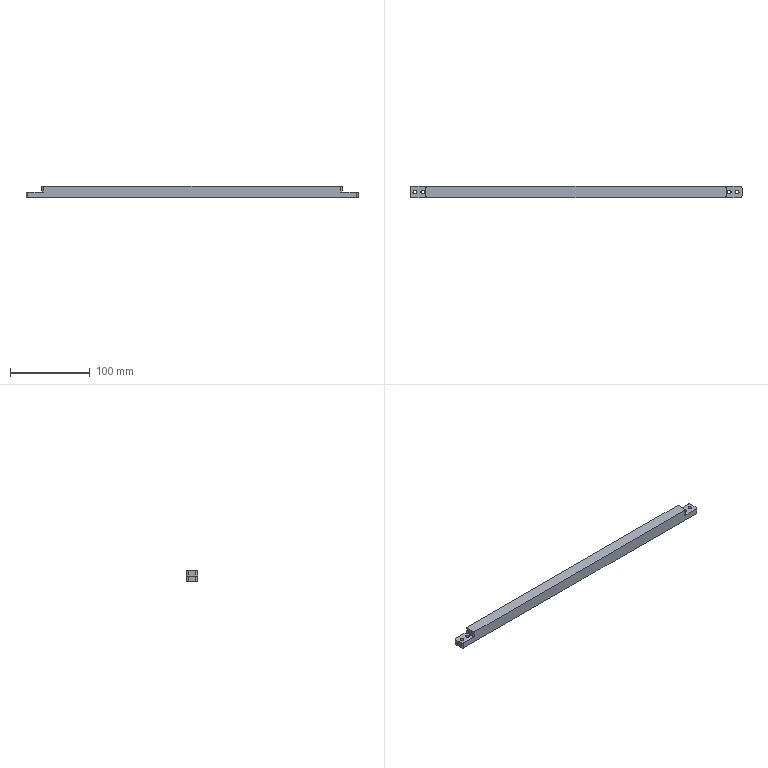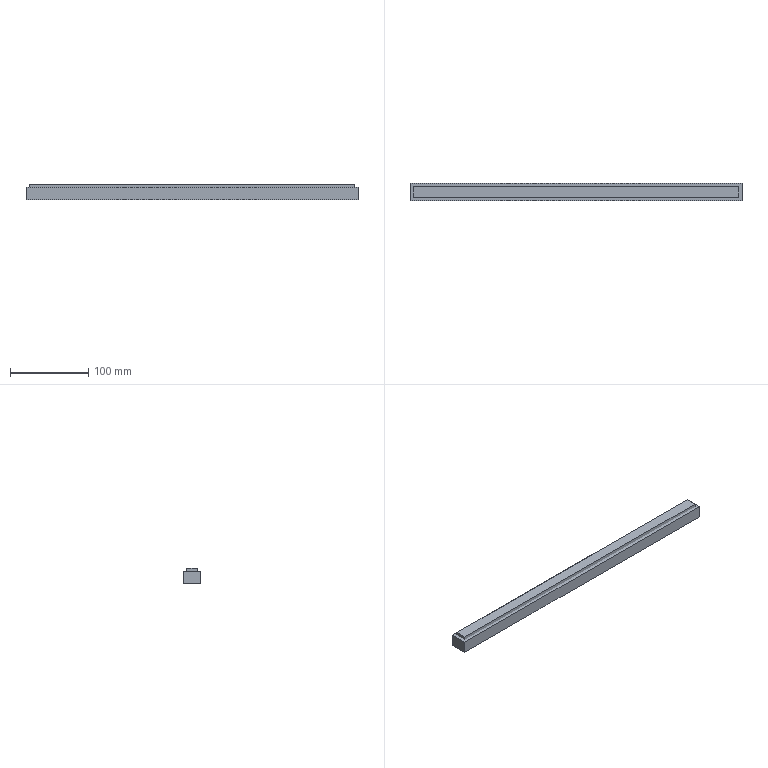CAM job | NX | 3-axis milling, drilling | part box 417 x 14 x 15 mm | stock box 425 x 22 x 20 mm
Tools:
number,name,description,diameter,corner_radius,flute_length,length,flutes
1,D63,Milling Tool-5 Parameters,63.0,0.0,50.0,75.0,2
2,D10,Milling Tool-5 Parameters,10.0,0.0,50.0,75.0,2
9,D6A45,Milling Tool-5 Parameters,6.0,0.0,3.0,3.0,2
10,2.5ZT,Drilling Tool,2.4,0.0,35.0,50.0,2
14,4.5ZT,Drilling Tool,4.5,0.0,35.0,50.0,2
4,D6,Milling Tool-5 Parameters,6.0,0.0,50.0,75.0,2
Operations:
program,operation,operation_type,tool,method,geometry_group,spindle_rpm,surface_speed,feed_per_tooth,feed_cut,feed_plunge,cut_length_mm,path_length_mm,cut_time_min,machine_time_min
1-425-20-20毛胚,FLOOR_WALL,VolumeBased25DMillingOperation,D63,METHOD,A,6500.0,0.0,0.0,1250.0,100.0,500.0,554.0,0.4,0.4054
1-425-20-20毛胚,ADAPTIVE_MILLING,CavityMilling,D10,METHOD,A,7000.0,219.0,0.1429,2000.0,1000.0,6258.453,6896.335,3.134,3.197
1-425-20-20毛胚,FLOOR_WALL_1_COPY_COPY_1_COPY,VolumeBased25DMillingOperation,D10,METHOD,A,7000.0,219.0,0.0714,1000.0,1000.0,332.091,1087.401,0.3321,0.4076
1-425-20-20毛胚,ZLEVEL_PROFILE_COPY_COPY_1_COPY,ZLevelMilling,D10,METHOD,A,6500.0,326.0,0.0769,1000.0,1000.0,899.046,986.046,0.899,0.9077
1-425-20-20毛胚,ZLEVEL_PROFILE_COPY_1_COPY_COPY_COPY_COPY,ZLevelMilling,D6A45,METHOD,A,7000.0,131.0,0.0714,1000.0,1000.0,787.53,849.53,0.7875,0.7937
1-425-20-20毛胚,ZLEVEL_PROFILE_COPY_1_COPY_COPY_COPY_COPY_COPY,ZLevelMilling,D6A45,METHOD,A,7000.0,131.0,0.0714,1000.0,1000.0,147.627,1421.552,0.1476,0.275
2-425-20-20毛胚,FLOOR_WALL_COPY,VolumeBased25DMillingOperation,D63,METHOD,B,6500.0,0.0,0.0,1250.0,100.0,2460.0,4654.001,1.968,2.187
2-425-20-20毛胚,DRILLING,Operation,D6A45,METHOD,B,4000.0,75.0,0.0312,250.0,0.0,48.0,596.027,0.192,0.2468
2-425-20-20毛胚,DRILLING_COPY_1,Operation,4.5ZT,METHOD,B,2000.0,20.0,0.05,200.0,0.0,53.408,581.708,0.267,0.3199
2-425-20-20毛胚,DRILLING_COPY_1_COPY,Operation,2.5ZT,METHOD,B,2000.0,20.0,0.05,120.0,0.0,93.679,618.987,0.7807,0.8332
2-425-20-20毛胚,HOLE_MILLING,CylinderMilling,D6,METHOD,B,7000.0,131.0,0.1214,1700.0,100.0,352.494,1013.494,0.2073,0.2734
2-425-20-20毛胚,ZLEVEL_PROFILE_COPY_1_COPY_COPY_COPY_COPY_COPY_1,ZLevelMilling,D6A45,METHOD,B,7000.0,131.0,0.0714,1000.0,1000.0,990.309,3314.181,0.9903,1.223